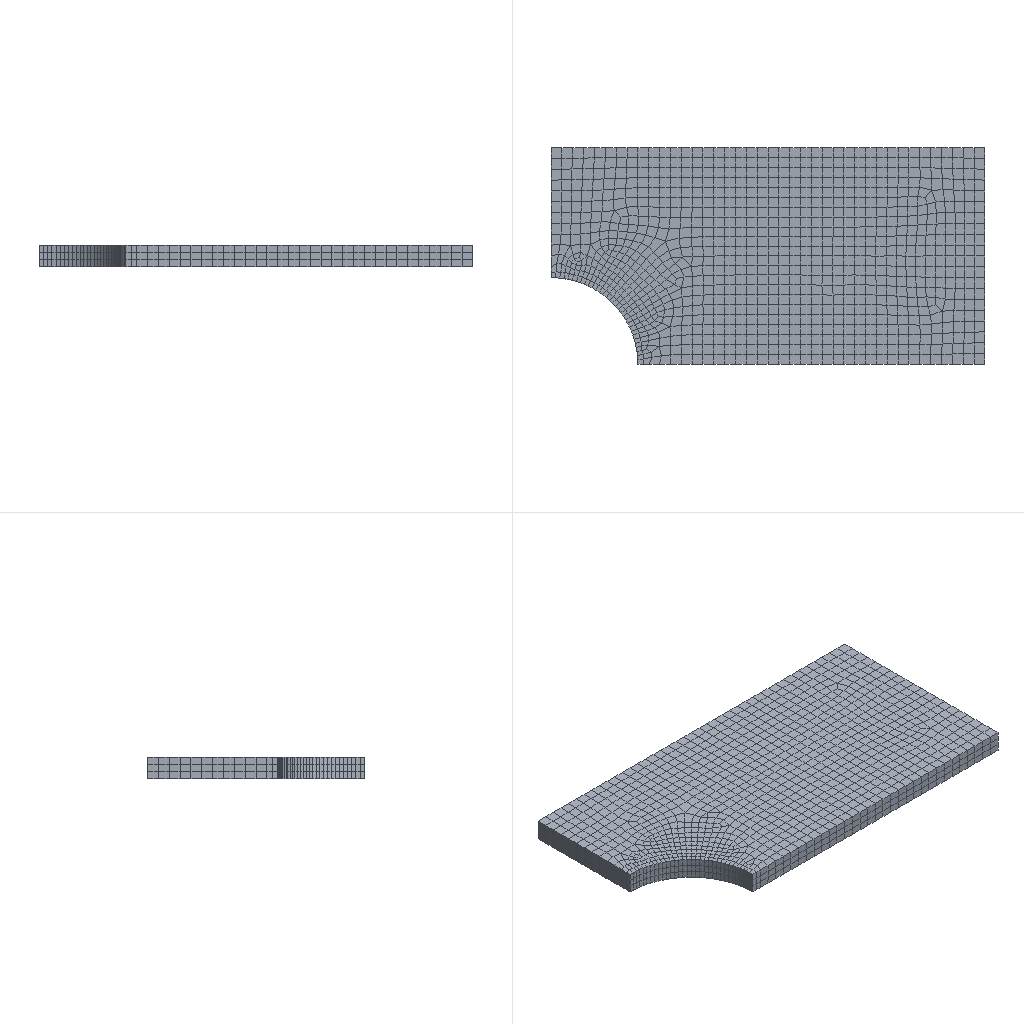Simulation study | ansys workbench
Set-up summary:
category,name,step,type,value,unit,region
solver,ansys_workbench
units,mm-N-s-tonne (MPa),,stated,"/units,MPA"
analysis,LS1,,static
load_step,LS1,LS1,static,nsubst=1; time=1
mesh,nodes,,,15125
mesh,elements,,,2934
element_type,SOLID186,,,2874
element_type,SURF154,,,60
material,Structural Steel,,E,200000,tonne s^-2 mm^-1
material,Structural Steel,,nu,0.3
material,Structural Steel,,density,7.85e-09,tonne mm^-3
material,Structural Steel,,conductivity,60.5,tonne mm s^-3 C^-1
material,Structural Steel,,specific_heat,4.34e+08,mm^2 s^-2 C^-1
material,Structural Steel,,cte,1.2e-05,C^-1
material,Structural Steel,,permeability,10000
material,Structural Steel,,resistivity,0.00017,ohm mm
load,Define Force Using Surface Effect Elements,LS1,surface-effect pres face 1,20,,SURF154 #2
bc,Frictionless Supports X,model,fixed,[dofs=UX],,_FRICSUX
bc,Frictionless Supports Y,model,fixed,[dofs=UY],,_FRICSUY
bc,Constant Zero Displacement Z,model,fixed,[dofs=UZ],,_DISPZEROUZ
named_set,_FRICSUX,,node,150
named_set,_FRICSUY,,node,370
named_set,_DISPZEROUZ,,node,3011
Ansys APDL input file, long lists of numbers shortened:
/batch
/config,noeldb,1     ! force off writing results to database
*get,_wallstrt,active,,time,wall
! ANSYS input file written by Workbench version 2021 R1
! File used for geometry attach:
/title,wbnew--____ (B5)
! ****** Begin Custom Load Command Snippet ******
/COM, ACT Extensions:
/COM,     LSDYNA, 2021.1
/COM,
! ****** End   Custom Load Command Snippet ******
*DIM,_wb_ProjectScratch_dir,string,248
_wb_ProjectScratch_dir(1) = ''
*DIM,_wb_SolverFiles_dir,string,248
_wb_SolverFiles_dir(1) = ''
*DIM,_wb_userfiles_dir,string,248
_wb_userfiles_dir(1) = ''
/com,--- Data in consistent NMM units. See Solving Units in the help system for more information.
/units,MPA
/nopr
/wb,file,start              !  signify a WB generated input file
/prep7
! Turn off shape checking because checks already performed inside WB mesher.
! See help system for more information.
SHPP,OFF,,NOWARN
/nolist
etcon,set             ! allow ANSYS to choose best KEYOP's for 180x elements, resets any applicable keyopt to MAPDL defaults
/com,*********** Nodes for the whole assembly ***********
nblock,3,,16637
(1i9,3e20.9e3)
        1     1.410832534E+01     2.623404520E+01     1.666666667E+00
! (15124 more lines like these left out)
-1
/wb,elem,start            !  set before creation of elements
/com,*********** Elements for Body 1 "2.1" ***********
et,1,186
keyo,1,2,1          ! set full integration on SOLID186
eblock,19,solid,,2874
(19i9)
        1        1        1        1        0        0        0        0       20        0        1      119     1557      121      187     2608     1889     2607     2574
! (5747 more lines like these left out)
-1
/wb,elem,end               !  done creating elements
/com,*********** Send User Defined Coordinate System(s) ***********
csys,0
toffst,273.15,  ! Temperature offset from absolute zero
/com,*********** Set Reference Temperature ***********
tref,22.
/wb,mat,start              !  starting to send materials
/com,*********** Send Materials ***********
Temperature = 'TEMP' ! Temperature
MP,DENS,1,7.85e-09,	! tonne mm^-3
MP,ALPX,1,1.2e-05,	! C^-1
MP,C,1,434000000,	! mm^2 s^-2 C^-1
MP,KXX,1,60.5,	! tonne mm s^-3 C^-1
MP,RSVX,1,0.00017,	! ohm mm
MP,EX,1,200000,	! tonne s^-2 mm^-1
MP,NUXY,1,0.3,
MP,MURX,1,10000,
/wb,mat,end                !  done sending materials
!************************* Model Summary ********************
!2.1,	结构钢,	matid,	1
!************************* End Model Summary ********************
! get the diagonal of the bounding box. Needed later for other things
*get,_xmin,node,,mnloc,x
*get,_ymin,node,,mnloc,y
*get,_zmin,node,,mnloc,z
*get,_xmax,node,,mxloc,x
*get,_ymax,node,,mxloc,y
*get,_zmax,node,,mxloc,z
_ASMDIAG=(_xmax-_xmin)*(_xmax-_xmin)+(_ymax-_ymin)*(_ymax-_ymin)+(_zmax-_zmin)*(_zmax-_zmin)
_ASMDIAG=SQRT(_ASMDIAG)
/wb,contact,start          !  starting to send contact
/wb,contact,end            !  done creating contacts
/golist
/wb,load,start             !  starting to send loads
/com,********* Frictionless Supports X *********
CMBLOCK,_FRICSUX,NODE,      150
(8i10)
      3557      3558      3559      3560      3561      3562      3563      3564
! (18 more lines like these left out)
cmsel,s,_FRICSUX
d,all,ux,0
nsel,all
/com,********* Frictionless Supports Y *********
CMBLOCK,_FRICSUY,NODE,      370
(8i10)
      3569      3570      3571      3572      3573      3574      3575      3576
! (46 more lines like these left out)
cmsel,s,_FRICSUY
d,all,uy,0
nsel,all
/com,******* Constant Zero Displacement Z *******
CMBLOCK,_DISPZEROUZ,NODE,     3011
(8i10)
      1779      1780      1781      1782      1783      1784      1785      1786
! (376 more lines like these left out)
cmsel,s,_DISPZEROUZ
d,all,uz,0
nsel,all
/com,*********** Define Force Using Surface Effect Elements ***********
local,12,0,0.,0.,0.,0.,0.,0.
csys,0
et,2,154
eblock,10,,,60
(15i9)
     5205        2        2        2       12     3976     3917     3619     3620    14814    14288    14287    14289
! (59 more lines like these left out)
-1
esel,s,type,,2
keyop,2,2,1                ! Apply load in local coordinate system
keyop,2,7,1                ! Use original area so load is constant in large deformation
esel,all
/gst,on,on
fini
*get,_numnode,node,0,count
*get,_numelem,elem,0,count
*get, _MAXELEMNUM, elem, 0, NUM, MAX
*get, _MAXNODENUM, node, 0, NUM, MAX
*get, _MAXELEMTYPE, etyp, 0, NUM, MAX
*get, _MAXREALCONST, real, 0, NUM, MAX
/go
/wb,load,end               !  done creating loads
/com,--- Number of total nodes = %_numnode%
/com,--- Number of contact elements = 60
/com,--- Number of spring elements = 0
/com,--- Number of bearing elements = 0
/com,--- Number of solid elements = 2874
/com,--- Number of condensed parts = 0
/com,--- Number of total elements = %_numelem%
*get,_wallbsol,active,,time,wall
/com,****************************************************************************
/com,*************************    SOLUTION       ********************************
/com,****************************************************************************
/solu
antype,0                   ! static analysis
_thickRatio=  1     ! Ratio of thick parts in the model
eqsl,pcg,1e-8,,,,,,1
cntr,print,1               ! print out contact info and also make no initial contact an error
dmpoption,emat,no             ! Don't combine emat file for DANSYS
dmpoption,esav,no             ! Don't combine esav file for DANSYS
nldiag,cont,iter           ! print out contact info each equilibrium iteration
rescontrol,,none                 ! Do not keep any restart files
/com,****************************************************
/com,******************* SOLVE FOR LS 1 OF 1 ****************
esel,s,type,,2
nsle
sfe,all,1,pres,1,20.
sfe,all,2,pres,1,0.
sfe,all,3,pres,1,0.
nsel,all
esel,all
/nopr
/gopr
/nolist
nsub,1,1,1
time,1.
outres,erase
outres,all,none
outres,nsol,all,
outres,rsol,all
outres,eangl,all
outres,etmp,all
outres,veng,all
outres,strs,all,
outres,epel,all,
outres,eppl,all,
outres,cont,all,
! *********** WB SOLVE COMMAND ***********
! check interactive state
*get,ANSINTER_,active,,int
*if,ANSINTER_,ne,0,then
/eof
*endif
solve
/com *************** Write FE CONNECTORS *********
CEWRITE,file,ce,,INTE
/com,****************************************************
/com,*************** FINISHED SOLVE FOR LS 1 *************
*get,_wallasol,active,,time,wall
/nopr
*get,_numnode,node,0,count
*get,_numelem,elem,0,count
*get, _MAXELEMNUM, elem, 0, NUM, MAX
*get, _MAXNODENUM, node, 0, NUM, MAX,,,INTERNAL
*get, _MAXELEMTYPE, etyp, 0, NUM, MAX
*get, _MAXREALCONST, real, 0, NUM, MAX
/gopr
*get,_PCGITER,active,,solu,cgiter
/post1
xmlo,ENCODING,ISO-8859-1
xmlo,parm
/xml,parm,xml
fini
/gopr
*get,_walldone,active,,time,wall
_preptime=(_wallbsol-_wallstrt)*3600
_solvtime=(_wallasol-_wallbsol)*3600
_posttime=(_walldone-_wallasol)*3600
_totaltim=(_walldone-_wallstrt)*3600
*get,_dlbratio,active,0,solu,dlbr
*get,_combtime,active,0,solu,comb
/com,--- Total number of nodes = %_numnode%
/com,--- Total number of elements = %_numelem%
/com,--- Element load balance ratio = %_dlbratio%
/com,--- Time to combine distributed files = %_combtime%
/wb,file,end               ! done with WB generated input
Results summary:
result,analyses[0].index,,,1
result,analyses[0].system,,,SYS-1
result,analyses[0].deck,,,deck.dat
result,analyses[0].solve_status,,,completed
result,analyses[0].analysis_type,,,static
result,analyses[0].physics,,,mechanical
result,analyses[0].unit_system,,,"NMM: mm, ton, N, s, mV, mA, degC"
result,analyses[0].n_sets,,,1
result,analyses[0].load_steps[0].set,set=1,,1
result,analyses[0].load_steps[0].time_or_freq,set=1,,1
result,analyses[0].load_steps[0].max_displacement_magnitude,set=1,,0.01258
result,analyses[0].load_steps[0].max_von_mises_nodal,set=1,,75.339
result,analyses[0].load_steps[0].reaction_force_sum_xyz[1],set=1,,-5000
result,analyses[0].load_steps[0].reaction_force_sum_xyz[2],set=1,,-1.40342e-05
result,analyses[0].load_steps[0].reaction_force_sum_xyz[3],set=1,,3.58399e-05
result,geometry_export[0][0],,,.step
result,geometry_export[0][1],,,ok
result,geometry_export[0][2],,,1